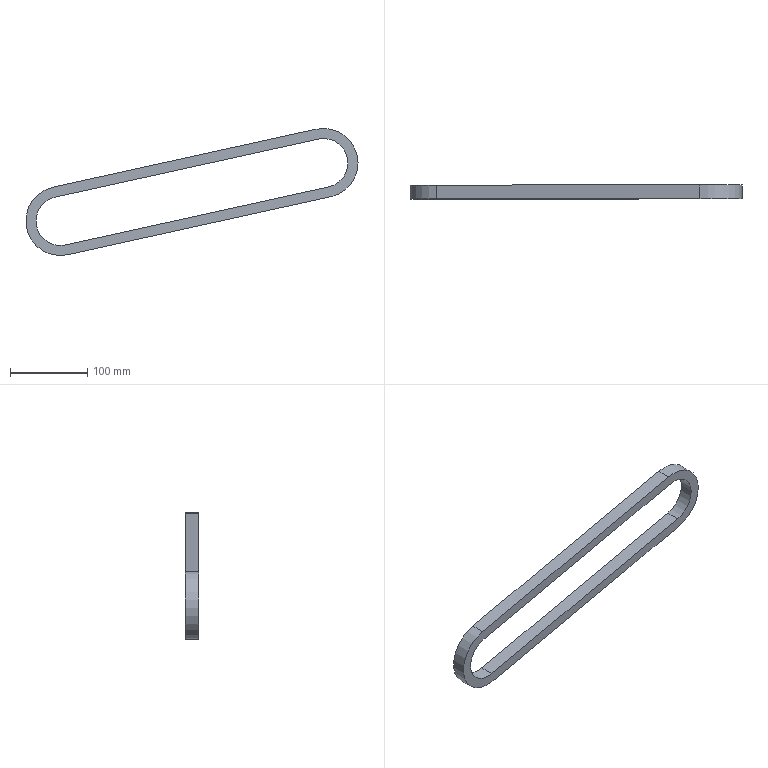Part | STEP file | CHAIN.stp | 1 solid | 12 faces | box 429.35 x 18 x 164.35 mm | volume 219073 mm3 | cylinder 6 | plane 6 | commonest cylinder face diameters 63.35 x3 89.35 x3
STEP:
#1=CARTESIAN_POINT('',(0.,0.,0.));
#2=DIRECTION('',(0.,0.,1.));
#3=DIRECTION('',(1.,0.,0.));
#4=AXIS2_PLACEMENT_3D('',#1,#2,#3);
#5=CARTESIAN_POINT('',(163.177,9.,68.431));
#6=VERTEX_POINT('',#5);
#7=CARTESIAN_POINT('',(163.177,-9.,68.431));
#8=VERTEX_POINT('',#7);
#9=CARTESIAN_POINT('',(163.177,9.,68.431));
#10=DIRECTION('',(0.,-1.,0.));
#11=VECTOR('',#10,1.);
#12=LINE('',#9,#11);
#13=CARTESIAN_POINT('',(170.,9.,37.5));
#14=DIRECTION('',(0.,-1.,0.));
#15=DIRECTION('',(1.,0.,0.));
#16=AXIS2_PLACEMENT_3D('',#13,#14,#15);
#17=CYLINDRICAL_SURFACE('',#16,31.675);
#18=CARTESIAN_POINT('',(1.788,0.));
#19=DIRECTION('',(0.,1.));
#20=VECTOR('',#19,1.);
#21=LINE('',#18,#20);
#22=(GEOMETRIC_REPRESENTATION_CONTEXT(2)PARAMETRIC_REPRESENTATION_CONTEXT()REPRESENTATION_CONTEXT('',''));
#23=DEFINITIONAL_REPRESENTATION('',(#21),#22);
#24=PCURVE('',#17,#23);
#25=CARTESIAN_POINT('',(163.177,9.,68.431));
#26=DIRECTION('',(0.2154,0.,-0.9765));
#27=DIRECTION('',(0.,-1.,0.));
#28=AXIS2_PLACEMENT_3D('',#25,#26,#27);
#29=PLANE('',#28);
#30=CARTESIAN_POINT('',(0.,0.));
#31=DIRECTION('',(1.,0.));
#32=VECTOR('',#31,1.);
#33=LINE('',#30,#32);
#34=(GEOMETRIC_REPRESENTATION_CONTEXT(2)PARAMETRIC_REPRESENTATION_CONTEXT()REPRESENTATION_CONTEXT('',''));
#35=DEFINITIONAL_REPRESENTATION('',(#33),#34);
#36=PCURVE('',#29,#35);
#37=SURFACE_CURVE('',#12,(#24,#36),.PCURVE_S1.);
#38=EDGE_CURVE('',#6,#8,#37,.T.);
#39=ORIENTED_EDGE('',*,*,#38,.T.);
#40=CARTESIAN_POINT('',(201.675,-9.,37.5));
#41=VERTEX_POINT('',#40);
#42=CARTESIAN_POINT('',(170.,-9.,37.5));
#43=DIRECTION('',(0.,-1.,0.));
#44=DIRECTION('',(1.,0.,0.));
#45=AXIS2_PLACEMENT_3D('',#42,#43,#44);
#46=CIRCLE('',#45,31.675);
#47=CARTESIAN_POINT('',(0.,18.));
#48=DIRECTION('',(1.,0.));
#49=VECTOR('',#48,1.);
#50=LINE('',#47,#49);
#51=(GEOMETRIC_REPRESENTATION_CONTEXT(2)PARAMETRIC_REPRESENTATION_CONTEXT()REPRESENTATION_CONTEXT('',''));
#52=DEFINITIONAL_REPRESENTATION('',(#50),#51);
#53=PCURVE('',#17,#52);
#54=CARTESIAN_POINT('',(0.,-9.,0.));
#55=DIRECTION('',(0.,1.,0.));
#56=DIRECTION('',(1.,0.,0.));
#57=AXIS2_PLACEMENT_3D('',#54,#55,#56);
#58=PLANE('',#57);
#59=CARTESIAN_POINT('',(201.675,-37.5));
#60=CARTESIAN_POINT('',(201.675,-92.363));
#61=CARTESIAN_POINT('',(154.162,-64.931));
#62=CARTESIAN_POINT('',(106.65,-37.5));
#63=CARTESIAN_POINT('',(154.162,-10.069));
#64=CARTESIAN_POINT('',(201.675,17.363));
#65=CARTESIAN_POINT('',(201.675,-37.5));
#66=(BOUNDED_CURVE()B_SPLINE_CURVE(2,(#59,#60,#61,#62,#63,#64,#65),.UNSPECIFIED.,.T.,.F.)B_SPLINE_CURVE_WITH_KNOTS((1,2,2,2,2,1),(-2.094,0.,2.094,4.189,6.283,8.378),.UNSPECIFIED.)CURVE()GEOMETRIC_REPRESENTATION_ITEM()RATIONAL_B_SPLINE_CURVE((1.,0.5,1.,0.5,1.,0.5,1.))REPRESENTATION_ITEM(''));
#67=(GEOMETRIC_REPRESENTATION_CONTEXT(2)PARAMETRIC_REPRESENTATION_CONTEXT()REPRESENTATION_CONTEXT('',''));
#68=DEFINITIONAL_REPRESENTATION('',(#66),#67);
#69=PCURVE('',#58,#68);
#70=SURFACE_CURVE('',#46,(#53,#69),.PCURVE_S1.);
#71=EDGE_CURVE('',#41,#8,#70,.T.);
#72=ORIENTED_EDGE('',*,*,#71,.F.);
#73=CARTESIAN_POINT('',(201.675,9.,37.5));
#74=VERTEX_POINT('',#73);
#75=CARTESIAN_POINT('',(201.675,9.,37.5));
#76=DIRECTION('',(0.,-1.,0.));
#77=VECTOR('',#76,1.);
#78=LINE('',#75,#77);
#79=CARTESIAN_POINT('',(0.,0.));
#80=DIRECTION('',(0.,1.));
#81=VECTOR('',#80,1.);
#82=LINE('',#79,#81);
#83=(GEOMETRIC_REPRESENTATION_CONTEXT(2)PARAMETRIC_REPRESENTATION_CONTEXT()REPRESENTATION_CONTEXT('',''));
#84=DEFINITIONAL_REPRESENTATION('',(#82),#83);
#85=PCURVE('',#17,#84);
#86=CARTESIAN_POINT('',(170.,9.,37.5));
#87=DIRECTION('',(0.,-1.,0.));
#88=DIRECTION('',(1.,0.,0.));
#89=AXIS2_PLACEMENT_3D('',#86,#87,#88);
#90=CYLINDRICAL_SURFACE('',#89,31.675);
#91=CARTESIAN_POINT('',(6.283,0.));
#92=DIRECTION('',(0.,1.));
#93=VECTOR('',#92,1.);
#94=LINE('',#91,#93);
#95=(GEOMETRIC_REPRESENTATION_CONTEXT(2)PARAMETRIC_REPRESENTATION_CONTEXT()REPRESENTATION_CONTEXT('',''));
#96=DEFINITIONAL_REPRESENTATION('',(#94),#95);
#97=PCURVE('',#90,#96);
#98=SURFACE_CURVE('',#78,(#85,#97),.PCURVE_S1.);
#99=EDGE_CURVE('',#74,#41,#98,.T.);
#100=ORIENTED_EDGE('',*,*,#99,.F.);
#101=CARTESIAN_POINT('',(170.,9.,37.5));
#102=DIRECTION('',(0.,1.,0.));
#103=DIRECTION('',(1.,0.,0.));
#104=AXIS2_PLACEMENT_3D('',#101,#102,#103);
#105=CIRCLE('',#104,31.675);
#106=CARTESIAN_POINT('',(6.283,0.));
#107=DIRECTION('',(-1.,0.));
#108=VECTOR('',#107,1.);
#109=LINE('',#106,#108);
#110=(GEOMETRIC_REPRESENTATION_CONTEXT(2)PARAMETRIC_REPRESENTATION_CONTEXT()REPRESENTATION_CONTEXT('',''));
#111=DEFINITIONAL_REPRESENTATION('',(#109),#110);
#112=PCURVE('',#17,#111);
#113=CARTESIAN_POINT('',(0.,9.,0.));
#114=DIRECTION('',(0.,1.,0.));
#115=DIRECTION('',(1.,0.,0.));
#116=AXIS2_PLACEMENT_3D('',#113,#114,#115);
#117=PLANE('',#116);
#118=CARTESIAN_POINT('',(170.,-37.5));
#119=DIRECTION('',(1.,0.));
#120=AXIS2_PLACEMENT_2D('',#118,#119);
#121=CIRCLE('',#120,31.675);
#122=(GEOMETRIC_REPRESENTATION_CONTEXT(2)PARAMETRIC_REPRESENTATION_CONTEXT()REPRESENTATION_CONTEXT('',''));
#123=DEFINITIONAL_REPRESENTATION('',(#121),#122);
#124=PCURVE('',#117,#123);
#125=SURFACE_CURVE('',#105,(#112,#124),.PCURVE_S1.);
#126=EDGE_CURVE('',#6,#74,#125,.T.);
#127=ORIENTED_EDGE('',*,*,#126,.F.);
#128=EDGE_LOOP('',(#39,#72,#100,#127));
#129=FACE_BOUND('',#128,.F.);
#130=ADVANCED_FACE('',(#129),#17,.F.);
#131=CARTESIAN_POINT('',(179.623,9.,-6.126));
#132=VERTEX_POINT('',#131);
#133=CARTESIAN_POINT('',(214.675,9.,37.5));
#134=VERTEX_POINT('',#133);
#135=CARTESIAN_POINT('',(170.,9.,37.5));
#136=DIRECTION('',(0.,-1.,0.));
#137=DIRECTION('',(1.,0.,0.));
#138=AXIS2_PLACEMENT_3D('',#135,#136,#137);
#139=CIRCLE('',#138,44.675);
#140=CARTESIAN_POINT('',(170.,9.,37.5));
#141=DIRECTION('',(0.,-1.,0.));
#142=DIRECTION('',(1.,0.,0.));
#143=AXIS2_PLACEMENT_3D('',#140,#141,#142);
#144=CYLINDRICAL_SURFACE('',#143,44.675);
#145=CARTESIAN_POINT('',(0.,0.));
#146=DIRECTION('',(1.,0.));
#147=VECTOR('',#146,1.);
#148=LINE('',#145,#147);
#149=(GEOMETRIC_REPRESENTATION_CONTEXT(2)PARAMETRIC_REPRESENTATION_CONTEXT()REPRESENTATION_CONTEXT('',''));
#150=DEFINITIONAL_REPRESENTATION('',(#148),#149);
#151=PCURVE('',#144,#150);
#152=CARTESIAN_POINT('',(214.675,-37.5));
#153=CARTESIAN_POINT('',(214.675,-114.879));
#154=CARTESIAN_POINT('',(147.662,-76.19));
#155=CARTESIAN_POINT('',(80.65,-37.5));
#156=CARTESIAN_POINT('',(147.662,1.19));
#157=CARTESIAN_POINT('',(214.675,39.879));
#158=CARTESIAN_POINT('',(214.675,-37.5));
#159=(BOUNDED_CURVE()B_SPLINE_CURVE(2,(#152,#153,#154,#155,#156,#157,#158),.UNSPECIFIED.,.T.,.F.)B_SPLINE_CURVE_WITH_KNOTS((1,2,2,2,2,1),(-2.094,0.,2.094,4.189,6.283,8.378),.UNSPECIFIED.)CURVE()GEOMETRIC_REPRESENTATION_ITEM()RATIONAL_B_SPLINE_CURVE((1.,0.5,1.,0.5,1.,0.5,1.))REPRESENTATION_ITEM(''));
#160=(GEOMETRIC_REPRESENTATION_CONTEXT(2)PARAMETRIC_REPRESENTATION_CONTEXT()REPRESENTATION_CONTEXT('',''));
#161=DEFINITIONAL_REPRESENTATION('',(#159),#160);
#162=PCURVE('',#117,#161);
#163=SURFACE_CURVE('',#139,(#151,#162),.PCURVE_S1.);
#164=EDGE_CURVE('',#132,#134,#163,.T.);
#165=ORIENTED_EDGE('',*,*,#164,.T.);
#166=CARTESIAN_POINT('',(214.675,-9.,37.5));
#167=VERTEX_POINT('',#166);
#168=CARTESIAN_POINT('',(214.675,9.,37.5));
#169=DIRECTION('',(0.,-1.,0.));
#170=VECTOR('',#169,1.);
#171=LINE('',#168,#170);
#172=CARTESIAN_POINT('',(6.283,0.));
#173=DIRECTION('',(0.,1.));
#174=VECTOR('',#173,1.);
#175=LINE('',#172,#174);
#176=(GEOMETRIC_REPRESENTATION_CONTEXT(2)PARAMETRIC_REPRESENTATION_CONTEXT()REPRESENTATION_CONTEXT('',''));
#177=DEFINITIONAL_REPRESENTATION('',(#175),#176);
#178=PCURVE('',#144,#177);
#179=CARTESIAN_POINT('',(170.,9.,37.5));
#180=DIRECTION('',(0.,-1.,0.));
#181=DIRECTION('',(1.,0.,0.));
#182=AXIS2_PLACEMENT_3D('',#179,#180,#181);
#183=CYLINDRICAL_SURFACE('',#182,44.675);
#184=CARTESIAN_POINT('',(0.,0.));
#185=DIRECTION('',(0.,1.));
#186=VECTOR('',#185,1.);
#187=LINE('',#184,#186);
#188=(GEOMETRIC_REPRESENTATION_CONTEXT(2)PARAMETRIC_REPRESENTATION_CONTEXT()REPRESENTATION_CONTEXT('',''));
#189=DEFINITIONAL_REPRESENTATION('',(#187),#188);
#190=PCURVE('',#183,#189);
#191=SURFACE_CURVE('',#171,(#178,#190),.PCURVE_S1.);
#192=EDGE_CURVE('',#134,#167,#191,.T.);
#193=ORIENTED_EDGE('',*,*,#192,.T.);
#194=CARTESIAN_POINT('',(179.623,-9.,-6.126));
#195=VERTEX_POINT('',#194);
#196=CARTESIAN_POINT('',(170.,-9.,37.5));
#197=DIRECTION('',(0.,1.,0.));
#198=DIRECTION('',(1.,0.,0.));
#199=AXIS2_PLACEMENT_3D('',#196,#197,#198);
#200=CIRCLE('',#199,44.675);
#201=CARTESIAN_POINT('',(6.283,18.));
#202=DIRECTION('',(-1.,0.));
#203=VECTOR('',#202,1.);
#204=LINE('',#201,#203);
#205=(GEOMETRIC_REPRESENTATION_CONTEXT(2)PARAMETRIC_REPRESENTATION_CONTEXT()REPRESENTATION_CONTEXT('',''));
#206=DEFINITIONAL_REPRESENTATION('',(#204),#205);
#207=PCURVE('',#144,#206);
#208=CARTESIAN_POINT('',(170.,-37.5));
#209=DIRECTION('',(1.,0.));
#210=AXIS2_PLACEMENT_2D('',#208,#209);
#211=CIRCLE('',#210,44.675);
#212=(GEOMETRIC_REPRESENTATION_CONTEXT(2)PARAMETRIC_REPRESENTATION_CONTEXT()REPRESENTATION_CONTEXT('',''));
#213=DEFINITIONAL_REPRESENTATION('',(#211),#212);
#214=PCURVE('',#58,#213);
#215=SURFACE_CURVE('',#200,(#207,#214),.PCURVE_S1.);
#216=EDGE_CURVE('',#167,#195,#215,.T.);
#217=ORIENTED_EDGE('',*,*,#216,.T.);
#218=CARTESIAN_POINT('',(179.623,9.,-6.126));
#219=DIRECTION('',(0.,-1.,0.));
#220=VECTOR('',#219,1.);
#221=LINE('',#218,#220);
#222=CARTESIAN_POINT('',(4.93,0.));
#223=DIRECTION('',(0.,1.));
#224=VECTOR('',#223,1.);
#225=LINE('',#222,#224);
#226=(GEOMETRIC_REPRESENTATION_CONTEXT(2)PARAMETRIC_REPRESENTATION_CONTEXT()REPRESENTATION_CONTEXT('',''));
#227=DEFINITIONAL_REPRESENTATION('',(#225),#226);
#228=PCURVE('',#144,#227);
#229=CARTESIAN_POINT('',(179.623,9.,-6.126));
#230=DIRECTION('',(0.2154,0.,-0.9765));
#231=DIRECTION('',(0.,-1.,0.));
#232=AXIS2_PLACEMENT_3D('',#229,#230,#231);
#233=PLANE('',#232);
#234=CARTESIAN_POINT('',(0.,0.));
#235=DIRECTION('',(1.,0.));
#236=VECTOR('',#235,1.);
#237=LINE('',#234,#236);
#238=(GEOMETRIC_REPRESENTATION_CONTEXT(2)PARAMETRIC_REPRESENTATION_CONTEXT()REPRESENTATION_CONTEXT('',''));
#239=DEFINITIONAL_REPRESENTATION('',(#237),#238);
#240=PCURVE('',#233,#239);
#241=SURFACE_CURVE('',#221,(#228,#240),.PCURVE_S1.);
#242=EDGE_CURVE('',#132,#195,#241,.T.);
#243=ORIENTED_EDGE('',*,*,#242,.F.);
#244=EDGE_LOOP('',(#165,#193,#217,#243));
#245=FACE_BOUND('',#244,.T.);
#246=ADVANCED_FACE('',(#245),#144,.T.);
#247=CARTESIAN_POINT('',(-176.823,9.,-6.569));
#248=VERTEX_POINT('',#247);
#249=CARTESIAN_POINT('',(-176.823,9.,-6.569));
#250=DIRECTION('',(0.9765,0.,0.2154));
#251=VECTOR('',#250,1.);
#252=LINE('',#249,#251);
#253=CARTESIAN_POINT('',(-176.823,6.569));
#254=DIRECTION('',(0.9765,-0.2154));
#255=VECTOR('',#254,1.);
#256=LINE('',#253,#255);
#257=(GEOMETRIC_REPRESENTATION_CONTEXT(2)PARAMETRIC_REPRESENTATION_CONTEXT()REPRESENTATION_CONTEXT('',''));
#258=DEFINITIONAL_REPRESENTATION('',(#256),#257);
#259=PCURVE('',#117,#258);
#260=CARTESIAN_POINT('',(0.,348.174));
#261=DIRECTION('',(0.,-1.));
#262=VECTOR('',#261,1.);
#263=LINE('',#260,#262);
#264=(GEOMETRIC_REPRESENTATION_CONTEXT(2)PARAMETRIC_REPRESENTATION_CONTEXT()REPRESENTATION_CONTEXT('',''));
#265=DEFINITIONAL_REPRESENTATION('',(#263),#264);
#266=PCURVE('',#29,#265);
#267=SURFACE_CURVE('',#252,(#259,#266),.PCURVE_S1.);
#268=EDGE_CURVE('',#248,#6,#267,.T.);
#269=ORIENTED_EDGE('',*,*,#268,.F.);
#270=CARTESIAN_POINT('',(-163.177,9.,-68.431));
#271=VERTEX_POINT('',#270);
#272=CARTESIAN_POINT('',(-170.,9.,-37.5));
#273=DIRECTION('',(0.,1.,0.));
#274=DIRECTION('',(1.,0.,0.));
#275=AXIS2_PLACEMENT_3D('',#272,#273,#274);
#276=CIRCLE('',#275,31.675);
#277=CARTESIAN_POINT('',(-170.,37.5));
#278=DIRECTION('',(1.,0.));
#279=AXIS2_PLACEMENT_2D('',#277,#278);
#280=CIRCLE('',#279,31.675);
#281=(GEOMETRIC_REPRESENTATION_CONTEXT(2)PARAMETRIC_REPRESENTATION_CONTEXT()REPRESENTATION_CONTEXT('',''));
#282=DEFINITIONAL_REPRESENTATION('',(#280),#281);
#283=PCURVE('',#117,#282);
#284=CARTESIAN_POINT('',(-170.,9.,-37.5));
#285=DIRECTION('',(0.,-1.,0.));
#286=DIRECTION('',(1.,0.,0.));
#287=AXIS2_PLACEMENT_3D('',#284,#285,#286);
#288=CYLINDRICAL_SURFACE('',#287,31.675);
#289=CARTESIAN_POINT('',(6.283,0.));
#290=DIRECTION('',(-1.,0.));
#291=VECTOR('',#290,1.);
#292=LINE('',#289,#291);
#293=(GEOMETRIC_REPRESENTATION_CONTEXT(2)PARAMETRIC_REPRESENTATION_CONTEXT()REPRESENTATION_CONTEXT('',''));
#294=DEFINITIONAL_REPRESENTATION('',(#292),#293);
#295=PCURVE('',#288,#294);
#296=SURFACE_CURVE('',#276,(#283,#295),.PCURVE_S1.);
#297=EDGE_CURVE('',#271,#248,#296,.T.);
#298=ORIENTED_EDGE('',*,*,#297,.F.);
#299=CARTESIAN_POINT('',(176.823,9.,6.569));
#300=VERTEX_POINT('',#299);
#301=CARTESIAN_POINT('',(176.823,9.,6.569));
#302=DIRECTION('',(-0.9765,0.,-0.2154));
#303=VECTOR('',#302,1.);
#304=LINE('',#301,#303);
#305=CARTESIAN_POINT('',(176.823,-6.569));
#306=DIRECTION('',(-0.9765,0.2154));
#307=VECTOR('',#306,1.);
#308=LINE('',#305,#307);
#309=(GEOMETRIC_REPRESENTATION_CONTEXT(2)PARAMETRIC_REPRESENTATION_CONTEXT()REPRESENTATION_CONTEXT('',''));
#310=DEFINITIONAL_REPRESENTATION('',(#308),#309);
#311=PCURVE('',#117,#310);
#312=CARTESIAN_POINT('',(-163.177,9.,-68.431));
#313=DIRECTION('',(-0.2154,0.,0.9765));
#314=DIRECTION('',(0.,1.,0.));
#315=AXIS2_PLACEMENT_3D('',#312,#313,#314);
#316=PLANE('',#315);
#317=CARTESIAN_POINT('',(0.,-348.174));
#318=DIRECTION('',(0.,1.));
#319=VECTOR('',#318,1.);
#320=LINE('',#317,#319);
#321=(GEOMETRIC_REPRESENTATION_CONTEXT(2)PARAMETRIC_REPRESENTATION_CONTEXT()REPRESENTATION_CONTEXT('',''));
#322=DEFINITIONAL_REPRESENTATION('',(#320),#321);
#323=PCURVE('',#316,#322);
#324=SURFACE_CURVE('',#304,(#311,#323),.PCURVE_S1.);
#325=EDGE_CURVE('',#300,#271,#324,.T.);
#326=ORIENTED_EDGE('',*,*,#325,.F.);
#327=CARTESIAN_POINT('',(170.,9.,37.5));
#328=DIRECTION('',(0.,1.,0.));
#329=DIRECTION('',(1.,0.,0.));
#330=AXIS2_PLACEMENT_3D('',#327,#328,#329);
#331=CIRCLE('',#330,31.675);
#332=CARTESIAN_POINT('',(170.,-37.5));
#333=DIRECTION('',(1.,0.));
#334=AXIS2_PLACEMENT_2D('',#332,#333);
#335=CIRCLE('',#334,31.675);
#336=(GEOMETRIC_REPRESENTATION_CONTEXT(2)PARAMETRIC_REPRESENTATION_CONTEXT()REPRESENTATION_CONTEXT('',''));
#337=DEFINITIONAL_REPRESENTATION('',(#335),#336);
#338=PCURVE('',#117,#337);
#339=CARTESIAN_POINT('',(6.283,0.));
#340=DIRECTION('',(-1.,0.));
#341=VECTOR('',#340,1.);
#342=LINE('',#339,#341);
#343=(GEOMETRIC_REPRESENTATION_CONTEXT(2)PARAMETRIC_REPRESENTATION_CONTEXT()REPRESENTATION_CONTEXT('',''));
#344=DEFINITIONAL_REPRESENTATION('',(#342),#343);
#345=PCURVE('',#90,#344);
#346=SURFACE_CURVE('',#331,(#338,#345),.PCURVE_S1.);
#347=EDGE_CURVE('',#74,#300,#346,.T.);
#348=ORIENTED_EDGE('',*,*,#347,.F.);
#349=ORIENTED_EDGE('',*,*,#126,.F.);
#350=EDGE_LOOP('',(#269,#298,#326,#348,#349));
#351=FACE_BOUND('',#350,.T.);
#352=CARTESIAN_POINT('',(-179.623,9.,6.126));
#353=VERTEX_POINT('',#352);
#354=CARTESIAN_POINT('',(160.377,9.,81.126));
#355=VERTEX_POINT('',#354);
#356=CARTESIAN_POINT('',(-179.623,9.,6.126));
#357=DIRECTION('',(0.9765,0.,0.2154));
#358=VECTOR('',#357,1.);
#359=LINE('',#356,#358);
#360=CARTESIAN_POINT('',(-179.623,-6.126));
#361=DIRECTION('',(0.9765,-0.2154));
#362=VECTOR('',#361,1.);
#363=LINE('',#360,#362);
#364=(GEOMETRIC_REPRESENTATION_CONTEXT(2)PARAMETRIC_REPRESENTATION_CONTEXT()REPRESENTATION_CONTEXT('',''));
#365=DEFINITIONAL_REPRESENTATION('',(#363),#364);
#366=PCURVE('',#117,#365);
#367=CARTESIAN_POINT('',(-179.623,9.,6.126));
#368=DIRECTION('',(-0.2154,0.,0.9765));
#369=DIRECTION('',(0.,1.,0.));
#370=AXIS2_PLACEMENT_3D('',#367,#368,#369);
#371=PLANE('',#370);
#372=CARTESIAN_POINT('',(0.,0.));
#373=DIRECTION('',(0.,-1.));
#374=VECTOR('',#373,1.);
#375=LINE('',#372,#374);
#376=(GEOMETRIC_REPRESENTATION_CONTEXT(2)PARAMETRIC_REPRESENTATION_CONTEXT()REPRESENTATION_CONTEXT('',''));
#377=DEFINITIONAL_REPRESENTATION('',(#375),#376);
#378=PCURVE('',#371,#377);
#379=SURFACE_CURVE('',#359,(#366,#378),.PCURVE_S1.);
#380=EDGE_CURVE('',#353,#355,#379,.T.);
#381=ORIENTED_EDGE('',*,*,#380,.T.);
#382=CARTESIAN_POINT('',(170.,9.,37.5));
#383=DIRECTION('',(0.,-1.,0.));
#384=DIRECTION('',(1.,0.,0.));
#385=AXIS2_PLACEMENT_3D('',#382,#383,#384);
#386=CIRCLE('',#385,44.675);
#387=CARTESIAN_POINT('',(214.675,-37.5));
#388=CARTESIAN_POINT('',(214.675,-114.879));
#389=CARTESIAN_POINT('',(147.662,-76.19));
#390=CARTESIAN_POINT('',(80.65,-37.5));
#391=CARTESIAN_POINT('',(147.662,1.19));
#392=CARTESIAN_POINT('',(214.675,39.879));
#393=CARTESIAN_POINT('',(214.675,-37.5));
#394=(BOUNDED_CURVE()B_SPLINE_CURVE(2,(#387,#388,#389,#390,#391,#392,#393),.UNSPECIFIED.,.T.,.F.)B_SPLINE_CURVE_WITH_KNOTS((1,2,2,2,2,1),(-2.094,0.,2.094,4.189,6.283,8.378),.UNSPECIFIED.)CURVE()GEOMETRIC_REPRESENTATION_ITEM()RATIONAL_B_SPLINE_CURVE((1.,0.5,1.,0.5,1.,0.5,1.))REPRESENTATION_ITEM(''));
#395=(GEOMETRIC_REPRESENTATION_CONTEXT(2)PARAMETRIC_REPRESENTATION_CONTEXT()REPRESENTATION_CONTEXT('',''));
#396=DEFINITIONAL_REPRESENTATION('',(#394),#395);
#397=PCURVE('',#117,#396);
#398=CARTESIAN_POINT('',(0.,0.));
#399=DIRECTION('',(1.,0.));
#400=VECTOR('',#399,1.);
#401=LINE('',#398,#400);
#402=(GEOMETRIC_REPRESENTATION_CONTEXT(2)PARAMETRIC_REPRESENTATION_CONTEXT()REPRESENTATION_CONTEXT('',''));
#403=DEFINITIONAL_REPRESENTATION('',(#401),#402);
#404=PCURVE('',#183,#403);
#405=SURFACE_CURVE('',#386,(#397,#404),.PCURVE_S1.);
#406=EDGE_CURVE('',#134,#355,#405,.T.);
#407=ORIENTED_EDGE('',*,*,#406,.F.);
#408=ORIENTED_EDGE('',*,*,#164,.F.);
#409=CARTESIAN_POINT('',(-160.377,9.,-81.126));
#410=VERTEX_POINT('',#409);
#411=CARTESIAN_POINT('',(-160.377,9.,-81.126));
#412=DIRECTION('',(0.9765,0.,0.2154));
#413=VECTOR('',#412,1.);
#414=LINE('',#411,#413);
#415=CARTESIAN_POINT('',(-160.377,81.126));
#416=DIRECTION('',(0.9765,-0.2154));
#417=VECTOR('',#416,1.);
#418=LINE('',#415,#417);
#419=(GEOMETRIC_REPRESENTATION_CONTEXT(2)PARAMETRIC_REPRESENTATION_CONTEXT()REPRESENTATION_CONTEXT('',''));
#420=DEFINITIONAL_REPRESENTATION('',(#418),#419);
#421=PCURVE('',#117,#420);
#422=CARTESIAN_POINT('',(0.,348.174));
#423=DIRECTION('',(0.,-1.));
#424=VECTOR('',#423,1.);
#425=LINE('',#422,#424);
#426=(GEOMETRIC_REPRESENTATION_CONTEXT(2)PARAMETRIC_REPRESENTATION_CONTEXT()REPRESENTATION_CONTEXT('',''));
#427=DEFINITIONAL_REPRESENTATION('',(#425),#426);
#428=PCURVE('',#233,#427);
#429=SURFACE_CURVE('',#414,(#421,#428),.PCURVE_S1.);
#430=EDGE_CURVE('',#410,#132,#429,.T.);
#431=ORIENTED_EDGE('',*,*,#430,.F.);
#432=CARTESIAN_POINT('',(-170.,9.,-37.5));
#433=DIRECTION('',(0.,-1.,0.));
#434=DIRECTION('',(1.,0.,0.));
#435=AXIS2_PLACEMENT_3D('',#432,#433,#434);
#436=CIRCLE('',#435,44.675);
#437=CARTESIAN_POINT('',(-125.325,37.5));
#438=CARTESIAN_POINT('',(-125.325,-39.879));
#439=CARTESIAN_POINT('',(-192.338,-1.19));
#440=CARTESIAN_POINT('',(-259.35,37.5));
#441=CARTESIAN_POINT('',(-192.338,76.19));
#442=CARTESIAN_POINT('',(-125.325,114.879));
#443=CARTESIAN_POINT('',(-125.325,37.5));
#444=(BOUNDED_CURVE()B_SPLINE_CURVE(2,(#437,#438,#439,#440,#441,#442,#443),.UNSPECIFIED.,.T.,.F.)B_SPLINE_CURVE_WITH_KNOTS((1,2,2,2,2,1),(-2.094,0.,2.094,4.189,6.283,8.378),.UNSPECIFIED.)CURVE()GEOMETRIC_REPRESENTATION_ITEM()RATIONAL_B_SPLINE_CURVE((1.,0.5,1.,0.5,1.,0.5,1.))REPRESENTATION_ITEM(''));
#445=(GEOMETRIC_REPRESENTATION_CONTEXT(2)PARAMETRIC_REPRESENTATION_CONTEXT()REPRESENTATION_CONTEXT('',''));
#446=DEFINITIONAL_REPRESENTATION('',(#444),#445);
#447=PCURVE('',#117,#446);
#448=CARTESIAN_POINT('',(-170.,9.,-37.5));
#449=DIRECTION('',(0.,-1.,0.));
#450=DIRECTION('',(1.,0.,0.));
#451=AXIS2_PLACEMENT_3D('',#448,#449,#450);
#452=CYLINDRICAL_SURFACE('',#451,44.675);
#453=CARTESIAN_POINT('',(0.,0.));
#454=DIRECTION('',(1.,0.));
#455=VECTOR('',#454,1.);
#456=LINE('',#453,#455);
#457=(GEOMETRIC_REPRESENTATION_CONTEXT(2)PARAMETRIC_REPRESENTATION_CONTEXT()REPRESENTATION_CONTEXT('',''));
#458=DEFINITIONAL_REPRESENTATION('',(#456),#457);
#459=PCURVE('',#452,#458);
#460=SURFACE_CURVE('',#436,(#447,#459),.PCURVE_S1.);
#461=EDGE_CURVE('',#353,#410,#460,.T.);
#462=ORIENTED_EDGE('',*,*,#461,.F.);
#463=EDGE_LOOP('',(#381,#407,#408,#431,#462));
#464=FACE_BOUND('',#463,.T.);
#465=ADVANCED_FACE('',(#351,#464),#117,.T.);
#466=CARTESIAN_POINT('',(-176.823,-9.,-6.569));
#467=VERTEX_POINT('',#466);
#468=CARTESIAN_POINT('',(-163.177,-9.,-68.431));
#469=VERTEX_POINT('',#468);
#470=CARTESIAN_POINT('',(-170.,-9.,-37.5));
#471=DIRECTION('',(0.,-1.,0.));
#472=DIRECTION('',(1.,0.,0.));
#473=AXIS2_PLACEMENT_3D('',#470,#471,#472);
#474=CIRCLE('',#473,31.675);
#475=CARTESIAN_POINT('',(-138.325,37.5));
#476=CARTESIAN_POINT('',(-138.325,-17.363));
#477=CARTESIAN_POINT('',(-185.838,10.069));
#478=CARTESIAN_POINT('',(-233.35,37.5));
#479=CARTESIAN_POINT('',(-185.838,64.931));
#480=CARTESIAN_POINT('',(-138.325,92.363));
#481=CARTESIAN_POINT('',(-138.325,37.5));
#482=(BOUNDED_CURVE()B_SPLINE_CURVE(2,(#475,#476,#477,#478,#479,#480,#481),.UNSPECIFIED.,.T.,.F.)B_SPLINE_CURVE_WITH_KNOTS((1,2,2,2,2,1),(-2.094,0.,2.094,4.189,6.283,8.378),.UNSPECIFIED.)CURVE()GEOMETRIC_REPRESENTATION_ITEM()RATIONAL_B_SPLINE_CURVE((1.,0.5,1.,0.5,1.,0.5,1.))REPRESENTATION_ITEM(''));
#483=(GEOMETRIC_REPRESENTATION_CONTEXT(2)PARAMETRIC_REPRESENTATION_CONTEXT()REPRESENTATION_CONTEXT('',''));
#484=DEFINITIONAL_REPRESENTATION('',(#482),#483);
#485=PCURVE('',#58,#484);
#486=CARTESIAN_POINT('',(0.,18.));
#487=DIRECTION('',(1.,0.));
#488=VECTOR('',#487,1.);
#489=LINE('',#486,#488);
#490=(GEOMETRIC_REPRESENTATION_CONTEXT(2)PARAMETRIC_REPRESENTATION_CONTEXT()REPRESENTATION_CONTEXT('',''));
#491=DEFINITIONAL_REPRESENTATION('',(#489),#490);
#492=PCURVE('',#288,#491);
#493=SURFACE_CURVE('',#474,(#485,#492),.PCURVE_S1.);
#494=EDGE_CURVE('',#467,#469,#493,.T.);
#495=ORIENTED_EDGE('',*,*,#494,.F.);
#496=CARTESIAN_POINT('',(163.177,-9.,68.431));
#497=DIRECTION('',(-0.9765,0.,-0.2154));
#498=VECTOR('',#497,1.);
#499=LINE('',#496,#498);
#500=CARTESIAN_POINT('',(163.177,-68.431));
#501=DIRECTION('',(-0.9765,0.2154));
#502=VECTOR('',#501,1.);
#503=LINE('',#500,#502);
#504=(GEOMETRIC_REPRESENTATION_CONTEXT(2)PARAMETRIC_REPRESENTATION_CONTEXT()REPRESENTATION_CONTEXT('',''));
#505=DEFINITIONAL_REPRESENTATION('',(#503),#504);
#506=PCURVE('',#58,#505);
#507=CARTESIAN_POINT('',(18.,0.));
#508=DIRECTION('',(0.,1.));
#509=VECTOR('',#508,1.);
#510=LINE('',#507,#509);
#511=(GEOMETRIC_REPRESENTATION_CONTEXT(2)PARAMETRIC_REPRESENTATION_CONTEXT()REPRESENTATION_CONTEXT('',''));
#512=DEFINITIONAL_REPRESENTATION('',(#510),#511);
#513=PCURVE('',#29,#512);
#514=SURFACE_CURVE('',#499,(#506,#513),.PCURVE_S1.);
#515=EDGE_CURVE('',#8,#467,#514,.T.);
#516=ORIENTED_EDGE('',*,*,#515,.F.);
#517=ORIENTED_EDGE('',*,*,#71,.F.);
#518=CARTESIAN_POINT('',(176.823,-9.,6.569));
#519=VERTEX_POINT('',#518);
#520=CARTESIAN_POINT('',(170.,-9.,37.5));
#521=DIRECTION('',(0.,-1.,0.));
#522=DIRECTION('',(1.,0.,0.));
#523=AXIS2_PLACEMENT_3D('',#520,#521,#522);
#524=CIRCLE('',#523,31.675);
#525=CARTESIAN_POINT('',(201.675,-37.5));
#526=CARTESIAN_POINT('',(201.675,-92.363));
#527=CARTESIAN_POINT('',(154.162,-64.931));
#528=CARTESIAN_POINT('',(106.65,-37.5));
#529=CARTESIAN_POINT('',(154.162,-10.069));
#530=CARTESIAN_POINT('',(201.675,17.363));
#531=CARTESIAN_POINT('',(201.675,-37.5));
#532=(BOUNDED_CURVE()B_SPLINE_CURVE(2,(#525,#526,#527,#528,#529,#530,#531),.UNSPECIFIED.,.T.,.F.)B_SPLINE_CURVE_WITH_KNOTS((1,2,2,2,2,1),(-2.094,0.,2.094,4.189,6.283,8.378),.UNSPECIFIED.)CURVE()GEOMETRIC_REPRESENTATION_ITEM()RATIONAL_B_SPLINE_CURVE((1.,0.5,1.,0.5,1.,0.5,1.))REPRESENTATION_ITEM(''));
#533=(GEOMETRIC_REPRESENTATION_CONTEXT(2)PARAMETRIC_REPRESENTATION_CONTEXT()REPRESENTATION_CONTEXT('',''));
#534=DEFINITIONAL_REPRESENTATION('',(#532),#533);
#535=PCURVE('',#58,#534);
#536=CARTESIAN_POINT('',(0.,18.));
#537=DIRECTION('',(1.,0.));
#538=VECTOR('',#537,1.);
#539=LINE('',#536,#538);
#540=(GEOMETRIC_REPRESENTATION_CONTEXT(2)PARAMETRIC_REPRESENTATION_CONTEXT()REPRESENTATION_CONTEXT('',''));
#541=DEFINITIONAL_REPRESENTATION('',(#539),#540);
#542=PCURVE('',#90,#541);
#543=SURFACE_CURVE('',#524,(#535,#542),.PCURVE_S1.);
#544=EDGE_CURVE('',#519,#41,#543,.T.);
#545=ORIENTED_EDGE('',*,*,#544,.F.);
#546=CARTESIAN_POINT('',(-163.177,-9.,-68.431));
#547=DIRECTION('',(0.9765,0.,0.2154));
#548=VECTOR('',#547,1.);
#549=LINE('',#546,#548);
#550=CARTESIAN_POINT('',(-163.177,68.431));
#551=DIRECTION('',(0.9765,-0.2154));
#552=VECTOR('',#551,1.);
#553=LINE('',#550,#552);
#554=(GEOMETRIC_REPRESENTATION_CONTEXT(2)PARAMETRIC_REPRESENTATION_CONTEXT()REPRESENTATION_CONTEXT('',''));
#555=DEFINITIONAL_REPRESENTATION('',(#553),#554);
#556=PCURVE('',#58,#555);
#557=CARTESIAN_POINT('',(-18.,0.));
#558=DIRECTION('',(0.,-1.));
#559=VECTOR('',#558,1.);
#560=LINE('',#557,#559);
#561=(GEOMETRIC_REPRESENTATION_CONTEXT(2)PARAMETRIC_REPRESENTATION_CONTEXT()REPRESENTATION_CONTEXT('',''));
#562=DEFINITIONAL_REPRESENTATION('',(#560),#561);
#563=PCURVE('',#316,#562);
#564=SURFACE_CURVE('',#549,(#556,#563),.PCURVE_S1.);
#565=EDGE_CURVE('',#469,#519,#564,.T.);
#566=ORIENTED_EDGE('',*,*,#565,.F.);
#567=EDGE_LOOP('',(#495,#516,#517,#545,#566));
#568=FACE_BOUND('',#567,.T.);
#569=CARTESIAN_POINT('',(160.377,-9.,81.126));
#570=VERTEX_POINT('',#569);
#571=CARTESIAN_POINT('',(170.,-9.,37.5));
#572=DIRECTION('',(0.,1.,0.));
#573=DIRECTION('',(1.,0.,0.));
#574=AXIS2_PLACEMENT_3D('',#571,#572,#573);
#575=CIRCLE('',#574,44.675);
#576=CARTESIAN_POINT('',(170.,-37.5));
#577=DIRECTION('',(1.,0.));
#578=AXIS2_PLACEMENT_2D('',#576,#577);
#579=CIRCLE('',#578,44.675);
#580=(GEOMETRIC_REPRESENTATION_CONTEXT(2)PARAMETRIC_REPRESENTATION_CONTEXT()REPRESENTATION_CONTEXT('',''));
#581=DEFINITIONAL_REPRESENTATION('',(#579),#580);
#582=PCURVE('',#58,#581);
#583=CARTESIAN_POINT('',(6.283,18.));
#584=DIRECTION('',(-1.,0.));
#585=VECTOR('',#584,1.);
#586=LINE('',#583,#585);
#587=(GEOMETRIC_REPRESENTATION_CONTEXT(2)PARAMETRIC_REPRESENTATION_CONTEXT()REPRESENTATION_CONTEXT('',''));
#588=DEFINITIONAL_REPRESENTATION('',(#586),#587);
#589=PCURVE('',#183,#588);
#590=SURFACE_CURVE('',#575,(#582,#589),.PCURVE_S1.);
#591=EDGE_CURVE('',#570,#167,#590,.T.);
#592=ORIENTED_EDGE('',*,*,#591,.F.);
#593=CARTESIAN_POINT('',(-179.623,-9.,6.126));
#594=VERTEX_POINT('',#593);
#595=CARTESIAN_POINT('',(-179.623,-9.,6.126));
#596=DIRECTION('',(0.9765,0.,0.2154));
#597=VECTOR('',#596,1.);
#598=LINE('',#595,#597);
#599=CARTESIAN_POINT('',(-179.623,-6.126));
#600=DIRECTION('',(0.9765,-0.2154));
#601=VECTOR('',#600,1.);
#602=LINE('',#599,#601);
#603=(GEOMETRIC_REPRESENTATION_CONTEXT(2)PARAMETRIC_REPRESENTATION_CONTEXT()REPRESENTATION_CONTEXT('',''));
#604=DEFINITIONAL_REPRESENTATION('',(#602),#603);
#605=PCURVE('',#58,#604);
#606=CARTESIAN_POINT('',(-18.,0.));
#607=DIRECTION('',(0.,-1.));
#608=VECTOR('',#607,1.);
#609=LINE('',#606,#608);
#610=(GEOMETRIC_REPRESENTATION_CONTEXT(2)PARAMETRIC_REPRESENTATION_CONTEXT()REPRESENTATION_CONTEXT('',''));
#611=DEFINITIONAL_REPRESENTATION('',(#609),#610);
#612=PCURVE('',#371,#611);
#613=SURFACE_CURVE('',#598,(#605,#612),.PCURVE_S1.);
#614=EDGE_CURVE('',#594,#570,#613,.T.);
#615=ORIENTED_EDGE('',*,*,#614,.F.);
#616=CARTESIAN_POINT('',(-160.377,-9.,-81.126));
#617=VERTEX_POINT('',#616);
#618=CARTESIAN_POINT('',(-170.,-9.,-37.5));
#619=DIRECTION('',(0.,1.,0.));
#620=DIRECTION('',(1.,0.,0.));
#621=AXIS2_PLACEMENT_3D('',#618,#619,#620);
#622=CIRCLE('',#621,44.675);
#623=CARTESIAN_POINT('',(-170.,37.5));
#624=DIRECTION('',(1.,0.));
#625=AXIS2_PLACEMENT_2D('',#623,#624);
#626=CIRCLE('',#625,44.675);
#627=(GEOMETRIC_REPRESENTATION_CONTEXT(2)PARAMETRIC_REPRESENTATION_CONTEXT()REPRESENTATION_CONTEXT('',''));
#628=DEFINITIONAL_REPRESENTATION('',(#626),#627);
#629=PCURVE('',#58,#628);
#630=CARTESIAN_POINT('',(6.283,18.));
#631=DIRECTION('',(-1.,0.));
#632=VECTOR('',#631,1.);
#633=LINE('',#630,#632);
#634=(GEOMETRIC_REPRESENTATION_CONTEXT(2)PARAMETRIC_REPRESENTATION_CONTEXT()REPRESENTATION_CONTEXT('',''));
#635=DEFINITIONAL_REPRESENTATION('',(#633),#634);
#636=PCURVE('',#452,#635);
#637=SURFACE_CURVE('',#622,(#629,#636),.PCURVE_S1.);
#638=EDGE_CURVE('',#617,#594,#637,.T.);
#639=ORIENTED_EDGE('',*,*,#638,.F.);
#640=CARTESIAN_POINT('',(179.623,-9.,-6.126));
#641=DIRECTION('',(-0.9765,0.,-0.2154));
#642=VECTOR('',#641,1.);
#643=LINE('',#640,#642);
#644=CARTESIAN_POINT('',(179.623,6.126));
#645=DIRECTION('',(-0.9765,0.2154));
#646=VECTOR('',#645,1.);
#647=LINE('',#644,#646);
#648=(GEOMETRIC_REPRESENTATION_CONTEXT(2)PARAMETRIC_REPRESENTATION_CONTEXT()REPRESENTATION_CONTEXT('',''));
#649=DEFINITIONAL_REPRESENTATION('',(#647),#648);
#650=PCURVE('',#58,#649);
#651=CARTESIAN_POINT('',(18.,0.));
#652=DIRECTION('',(0.,1.));
#653=VECTOR('',#652,1.);
#654=LINE('',#651,#653);
#655=(GEOMETRIC_REPRESENTATION_CONTEXT(2)PARAMETRIC_REPRESENTATION_CONTEXT()REPRESENTATION_CONTEXT('',''));
#656=DEFINITIONAL_REPRESENTATION('',(#654),#655);
#657=PCURVE('',#233,#656);
#658=SURFACE_CURVE('',#643,(#650,#657),.PCURVE_S1.);
#659=EDGE_CURVE('',#195,#617,#658,.T.);
#660=ORIENTED_EDGE('',*,*,#659,.F.);
#661=ORIENTED_EDGE('',*,*,#216,.F.);
#662=EDGE_LOOP('',(#592,#615,#639,#660,#661));
#663=FACE_BOUND('',#662,.T.);
#664=ADVANCED_FACE('',(#568,#663),#58,.F.);
#665=ORIENTED_EDGE('',*,*,#614,.T.);
#666=CARTESIAN_POINT('',(160.377,9.,81.126));
#667=DIRECTION('',(0.,-1.,0.));
#668=VECTOR('',#667,1.);
#669=LINE('',#666,#668);
#670=CARTESIAN_POINT('',(0.,-348.174));
#671=DIRECTION('',(-1.,0.));
#672=VECTOR('',#671,1.);
#673=LINE('',#670,#672);
#674=(GEOMETRIC_REPRESENTATION_CONTEXT(2)PARAMETRIC_REPRESENTATION_CONTEXT()REPRESENTATION_CONTEXT('',''));
#675=DEFINITIONAL_REPRESENTATION('',(#673),#674);
#676=PCURVE('',#371,#675);
#677=CARTESIAN_POINT('',(1.788,0.));
#678=DIRECTION('',(0.,1.));
#679=VECTOR('',#678,1.);
#680=LINE('',#677,#679);
#681=(GEOMETRIC_REPRESENTATION_CONTEXT(2)PARAMETRIC_REPRESENTATION_CONTEXT()REPRESENTATION_CONTEXT('',''));
#682=DEFINITIONAL_REPRESENTATION('',(#680),#681);
#683=PCURVE('',#183,#682);
#684=SURFACE_CURVE('',#669,(#676,#683),.PCURVE_S1.);
#685=EDGE_CURVE('',#355,#570,#684,.T.);
#686=ORIENTED_EDGE('',*,*,#685,.F.);
#687=ORIENTED_EDGE('',*,*,#380,.F.);
#688=CARTESIAN_POINT('',(-179.623,9.,6.126));
#689=DIRECTION('',(0.,-1.,0.));
#690=VECTOR('',#689,1.);
#691=LINE('',#688,#690);
#692=CARTESIAN_POINT('',(0.,0.));
#693=DIRECTION('',(-1.,0.));
#694=VECTOR('',#693,1.);
#695=LINE('',#692,#694);
#696=(GEOMETRIC_REPRESENTATION_CONTEXT(2)PARAMETRIC_REPRESENTATION_CONTEXT()REPRESENTATION_CONTEXT('',''));
#697=DEFINITIONAL_REPRESENTATION('',(#695),#696);
#698=PCURVE('',#371,#697);
#699=CARTESIAN_POINT('',(1.788,0.));
#700=DIRECTION('',(0.,1.));
#701=VECTOR('',#700,1.);
#702=LINE('',#699,#701);
#703=(GEOMETRIC_REPRESENTATION_CONTEXT(2)PARAMETRIC_REPRESENTATION_CONTEXT()REPRESENTATION_CONTEXT('',''));
#704=DEFINITIONAL_REPRESENTATION('',(#702),#703);
#705=PCURVE('',#452,#704);
#706=SURFACE_CURVE('',#691,(#698,#705),.PCURVE_S1.);
#707=EDGE_CURVE('',#353,#594,#706,.T.);
#708=ORIENTED_EDGE('',*,*,#707,.T.);
#709=EDGE_LOOP('',(#665,#686,#687,#708));
#710=FACE_BOUND('',#709,.T.);
#711=ADVANCED_FACE('',(#710),#371,.T.);
#712=ORIENTED_EDGE('',*,*,#638,.T.);
#713=ORIENTED_EDGE('',*,*,#707,.F.);
#714=ORIENTED_EDGE('',*,*,#461,.T.);
#715=CARTESIAN_POINT('',(-160.377,9.,-81.126));
#716=DIRECTION('',(0.,-1.,0.));
#717=VECTOR('',#716,1.);
#718=LINE('',#715,#717);
#719=CARTESIAN_POINT('',(4.93,0.));
#720=DIRECTION('',(0.,1.));
#721=VECTOR('',#720,1.);
#722=LINE('',#719,#721);
#723=(GEOMETRIC_REPRESENTATION_CONTEXT(2)PARAMETRIC_REPRESENTATION_CONTEXT()REPRESENTATION_CONTEXT('',''));
#724=DEFINITIONAL_REPRESENTATION('',(#722),#723);
#725=PCURVE('',#452,#724);
#726=CARTESIAN_POINT('',(0.,348.174));
#727=DIRECTION('',(1.,0.));
#728=VECTOR('',#727,1.);
#729=LINE('',#726,#728);
#730=(GEOMETRIC_REPRESENTATION_CONTEXT(2)PARAMETRIC_REPRESENTATION_CONTEXT()REPRESENTATION_CONTEXT('',''));
#731=DEFINITIONAL_REPRESENTATION('',(#729),#730);
#732=PCURVE('',#233,#731);
#733=SURFACE_CURVE('',#718,(#725,#732),.PCURVE_S1.);
#734=EDGE_CURVE('',#410,#617,#733,.T.);
#735=ORIENTED_EDGE('',*,*,#734,.T.);
#736=EDGE_LOOP('',(#712,#713,#714,#735));
#737=FACE_BOUND('',#736,.T.);
#738=ADVANCED_FACE('',(#737),#452,.T.);
#739=ORIENTED_EDGE('',*,*,#659,.T.);
#740=ORIENTED_EDGE('',*,*,#734,.F.);
#741=ORIENTED_EDGE('',*,*,#430,.T.);
#742=ORIENTED_EDGE('',*,*,#242,.T.);
#743=EDGE_LOOP('',(#739,#740,#741,#742));
#744=FACE_BOUND('',#743,.T.);
#745=ADVANCED_FACE('',(#744),#233,.T.);
#746=ORIENTED_EDGE('',*,*,#192,.F.);
#747=ORIENTED_EDGE('',*,*,#406,.T.);
#748=ORIENTED_EDGE('',*,*,#685,.T.);
#749=ORIENTED_EDGE('',*,*,#591,.T.);
#750=EDGE_LOOP('',(#746,#747,#748,#749));
#751=FACE_BOUND('',#750,.T.);
#752=ADVANCED_FACE('',(#751),#183,.T.);
#753=ORIENTED_EDGE('',*,*,#515,.T.);
#754=CARTESIAN_POINT('',(-176.823,9.,-6.569));
#755=DIRECTION('',(0.,-1.,0.));
#756=VECTOR('',#755,1.);
#757=LINE('',#754,#756);
#758=CARTESIAN_POINT('',(0.,348.174));
#759=DIRECTION('',(1.,0.));
#760=VECTOR('',#759,1.);
#761=LINE('',#758,#760);
#762=(GEOMETRIC_REPRESENTATION_CONTEXT(2)PARAMETRIC_REPRESENTATION_CONTEXT()REPRESENTATION_CONTEXT('',''));
#763=DEFINITIONAL_REPRESENTATION('',(#761),#762);
#764=PCURVE('',#29,#763);
#765=CARTESIAN_POINT('',(1.788,0.));
#766=DIRECTION('',(0.,1.));
#767=VECTOR('',#766,1.);
#768=LINE('',#765,#767);
#769=(GEOMETRIC_REPRESENTATION_CONTEXT(2)PARAMETRIC_REPRESENTATION_CONTEXT()REPRESENTATION_CONTEXT('',''));
#770=DEFINITIONAL_REPRESENTATION('',(#768),#769);
#771=PCURVE('',#288,#770);
#772=SURFACE_CURVE('',#757,(#764,#771),.PCURVE_S1.);
#773=EDGE_CURVE('',#248,#467,#772,.T.);
#774=ORIENTED_EDGE('',*,*,#773,.F.);
#775=ORIENTED_EDGE('',*,*,#268,.T.);
#776=ORIENTED_EDGE('',*,*,#38,.T.);
#777=EDGE_LOOP('',(#753,#774,#775,#776));
#778=FACE_BOUND('',#777,.T.);
#779=ADVANCED_FACE('',(#778),#29,.T.);
#780=ORIENTED_EDGE('',*,*,#544,.F.);
#781=CARTESIAN_POINT('',(176.823,9.,6.569));
#782=DIRECTION('',(0.,-1.,0.));
#783=VECTOR('',#782,1.);
#784=LINE('',#781,#783);
#785=CARTESIAN_POINT('',(4.93,0.));
#786=DIRECTION('',(0.,1.));
#787=VECTOR('',#786,1.);
#788=LINE('',#785,#787);
#789=(GEOMETRIC_REPRESENTATION_CONTEXT(2)PARAMETRIC_REPRESENTATION_CONTEXT()REPRESENTATION_CONTEXT('',''));
#790=DEFINITIONAL_REPRESENTATION('',(#788),#789);
#791=PCURVE('',#90,#790);
#792=CARTESIAN_POINT('',(0.,-348.174));
#793=DIRECTION('',(-1.,0.));
#794=VECTOR('',#793,1.);
#795=LINE('',#792,#794);
#796=(GEOMETRIC_REPRESENTATION_CONTEXT(2)PARAMETRIC_REPRESENTATION_CONTEXT()REPRESENTATION_CONTEXT('',''));
#797=DEFINITIONAL_REPRESENTATION('',(#795),#796);
#798=PCURVE('',#316,#797);
#799=SURFACE_CURVE('',#784,(#791,#798),.PCURVE_S1.);
#800=EDGE_CURVE('',#300,#519,#799,.T.);
#801=ORIENTED_EDGE('',*,*,#800,.F.);
#802=ORIENTED_EDGE('',*,*,#347,.F.);
#803=ORIENTED_EDGE('',*,*,#99,.T.);
#804=EDGE_LOOP('',(#780,#801,#802,#803));
#805=FACE_BOUND('',#804,.F.);
#806=ADVANCED_FACE('',(#805),#90,.F.);
#807=ORIENTED_EDGE('',*,*,#565,.T.);
#808=ORIENTED_EDGE('',*,*,#800,.F.);
#809=ORIENTED_EDGE('',*,*,#325,.T.);
#810=CARTESIAN_POINT('',(-163.177,9.,-68.431));
#811=DIRECTION('',(0.,-1.,0.));
#812=VECTOR('',#811,1.);
#813=LINE('',#810,#812);
#814=CARTESIAN_POINT('',(0.,0.));
#815=DIRECTION('',(-1.,0.));
#816=VECTOR('',#815,1.);
#817=LINE('',#814,#816);
#818=(GEOMETRIC_REPRESENTATION_CONTEXT(2)PARAMETRIC_REPRESENTATION_CONTEXT()REPRESENTATION_CONTEXT('',''));
#819=DEFINITIONAL_REPRESENTATION('',(#817),#818);
#820=PCURVE('',#316,#819);
#821=CARTESIAN_POINT('',(4.93,0.));
#822=DIRECTION('',(0.,1.));
#823=VECTOR('',#822,1.);
#824=LINE('',#821,#823);
#825=(GEOMETRIC_REPRESENTATION_CONTEXT(2)PARAMETRIC_REPRESENTATION_CONTEXT()REPRESENTATION_CONTEXT('',''));
#826=DEFINITIONAL_REPRESENTATION('',(#824),#825);
#827=PCURVE('',#288,#826);
#828=SURFACE_CURVE('',#813,(#820,#827),.PCURVE_S1.);
#829=EDGE_CURVE('',#271,#469,#828,.T.);
#830=ORIENTED_EDGE('',*,*,#829,.T.);
#831=EDGE_LOOP('',(#807,#808,#809,#830));
#832=FACE_BOUND('',#831,.T.);
#833=ADVANCED_FACE('',(#832),#316,.T.);
#834=ORIENTED_EDGE('',*,*,#773,.F.);
#835=ORIENTED_EDGE('',*,*,#297,.F.);
#836=ORIENTED_EDGE('',*,*,#829,.T.);
#837=ORIENTED_EDGE('',*,*,#494,.F.);
#838=EDGE_LOOP('',(#834,#835,#836,#837));
#839=FACE_BOUND('',#838,.F.);
#840=ADVANCED_FACE('',(#839),#288,.F.);
#841=CLOSED_SHELL('',(#130,#246,#465,#664,#711,#738,#745,#752,#779,#806,#833,#840));
#842=MANIFOLD_SOLID_BREP('',#841);
#843=(LENGTH_UNIT()NAMED_UNIT(*)SI_UNIT(.MILLI.,.METRE.));
#844=UNCERTAINTY_MEASURE_WITH_UNIT(LENGTH_MEASURE(0.0000001),#843,'','');
#845=(NAMED_UNIT(*)PLANE_ANGLE_UNIT()SI_UNIT($,.RADIAN.));
#846=(NAMED_UNIT(*)SI_UNIT($,.STERADIAN.)SOLID_ANGLE_UNIT());
#847=(GEOMETRIC_REPRESENTATION_CONTEXT(3)GLOBAL_UNCERTAINTY_ASSIGNED_CONTEXT((#844))GLOBAL_UNIT_ASSIGNED_CONTEXT((#843,#845,#846))REPRESENTATION_CONTEXT('',''));
#848=ADVANCED_BREP_SHAPE_REPRESENTATION('',(#4,#842),#847);